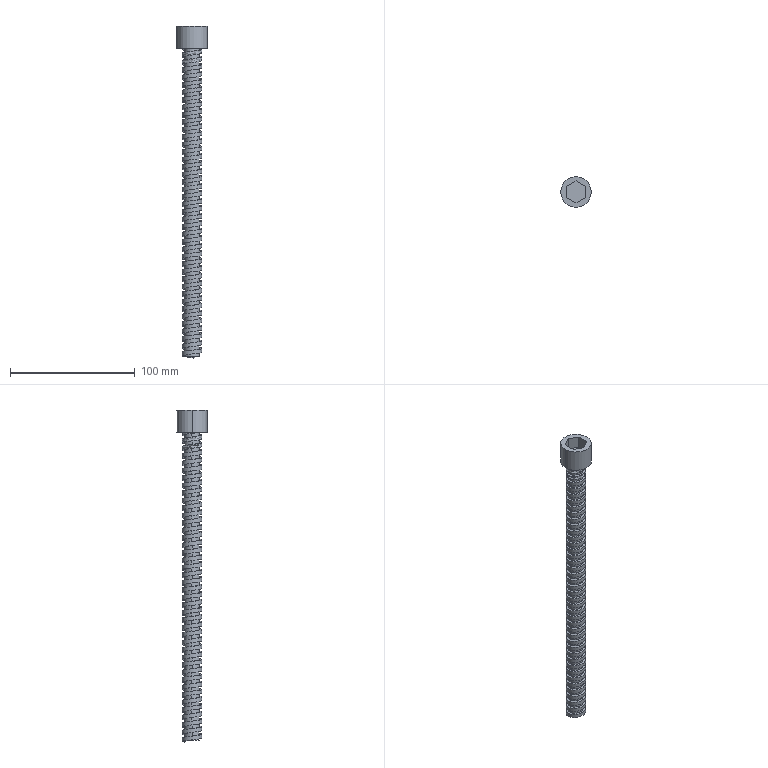Part | SolidWorks | features ICE 2, Extrusion 1, Helix 1, Sweep 1 | 1 solid | 102 faces | box 24.5 x 24.5 x 266.5 mm | volume 45236 mm3 | cylinder 87 | plane 11 | spline 4 | commonest cylinder face diameters 12 x85 24.5 x2